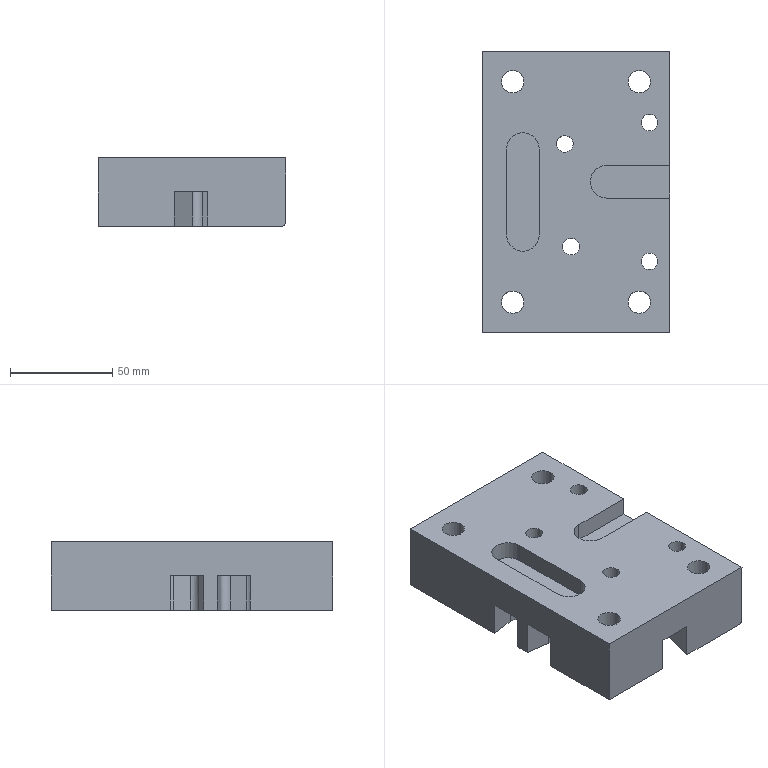Part | STEP file | gslz 2016.10.28-6_id1078_x_t | 1 solid | 83 faces | box 92 x 138 x 33.5 mm | volume 325352 mm3 | plane 39 | cylinder 35 | cone 5 | torus 4 | commonest cylinder face diameters 8 x8 4.5 x4 8.2 x4 10 x4 11 x4 17 x4